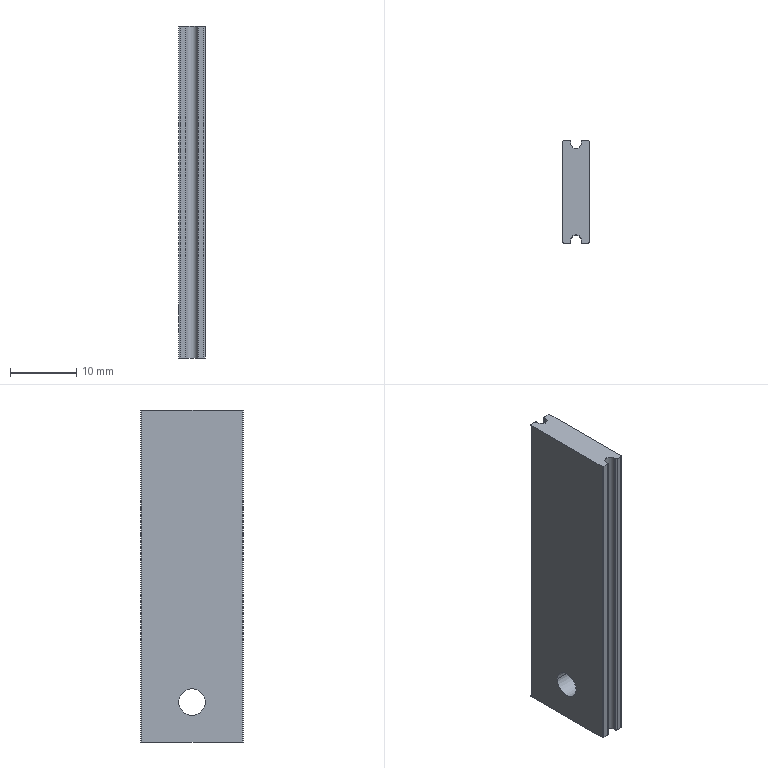Part | STEP file | CHAY 3.9 | 1 solid | 24 faces | box 4 x 15.5 x 50 mm | volume 2874 mm3 | cylinder 12 | plane 12 | commonest cylinder face diameters 0.4 x8 1.6 x2 4 x2